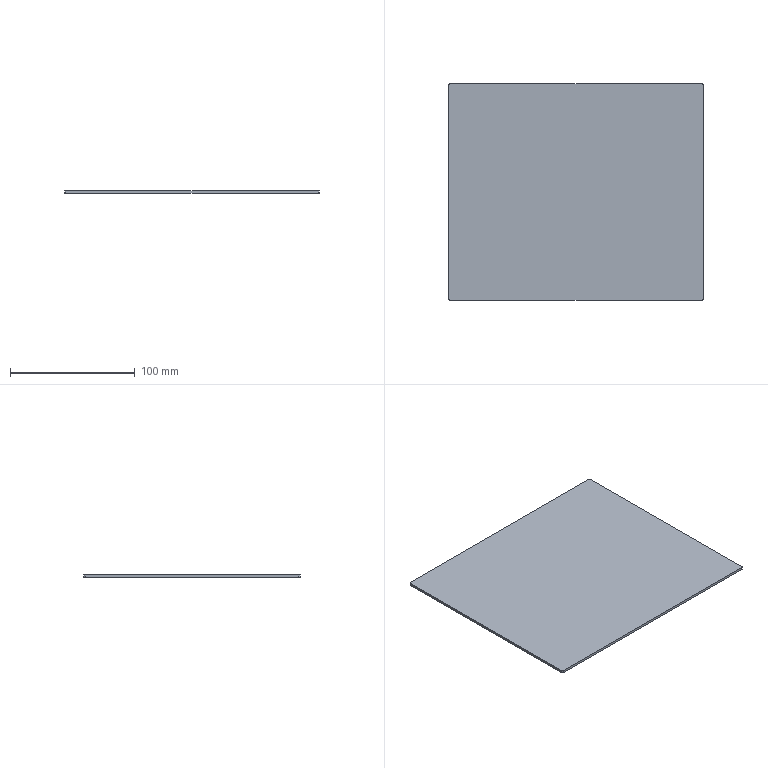Part | NX | features BREP 1 | 1 solid | 10 faces | box 204 x 173 x 2 mm | volume 70582 mm3 | plane 6 | cylinder 4 | commonest cylinder face diameters 2 x4
STEP:
#1=CARTESIAN_POINT('',(101.,86.5,-2.));
#2=VERTEX_POINT('',#1);
#3=CARTESIAN_POINT('',(-101.,86.5,-2.));
#4=VERTEX_POINT('',#3);
#5=CARTESIAN_POINT('',(-101.,86.5,-2.));
#6=DIRECTION('',(-1.,0.,0.));
#7=VECTOR('',#6,1000.);
#8=LINE('',#5,#7);
#9=EDGE_CURVE('',#2,#4,#8,.T.);
#10=ORIENTED_EDGE('',*,*,#9,.F.);
#11=CARTESIAN_POINT('',(102.,85.5,-2.));
#12=VERTEX_POINT('',#11);
#13=CARTESIAN_POINT('',(101.,85.5,-2.));
#14=DIRECTION('',(0.,0.,1.));
#15=DIRECTION('',(1.,0.,0.));
#16=AXIS2_PLACEMENT_3D('',#13,#14,#15);
#17=CIRCLE('',#16,1.);
#18=EDGE_CURVE('',#12,#2,#17,.T.);
#19=ORIENTED_EDGE('',*,*,#18,.F.);
#20=CARTESIAN_POINT('',(102.,-85.5,-2.));
#21=VERTEX_POINT('',#20);
#22=CARTESIAN_POINT('',(102.,-85.5,-2.));
#23=DIRECTION('',(0.,1.,0.));
#24=VECTOR('',#23,1000.);
#25=LINE('',#22,#24);
#26=EDGE_CURVE('',#21,#12,#25,.T.);
#27=ORIENTED_EDGE('',*,*,#26,.F.);
#28=CARTESIAN_POINT('',(101.,-86.5,-2.));
#29=VERTEX_POINT('',#28);
#30=CARTESIAN_POINT('',(101.,-85.5,-2.));
#31=DIRECTION('',(0.,0.,1.));
#32=DIRECTION('',(1.,0.,0.));
#33=AXIS2_PLACEMENT_3D('',#30,#31,#32);
#34=CIRCLE('',#33,1.);
#35=EDGE_CURVE('',#29,#21,#34,.T.);
#36=ORIENTED_EDGE('',*,*,#35,.F.);
#37=CARTESIAN_POINT('',(-101.,-86.5,-2.));
#38=VERTEX_POINT('',#37);
#39=CARTESIAN_POINT('',(-101.,-86.5,-2.));
#40=DIRECTION('',(1.,0.,0.));
#41=VECTOR('',#40,1000.);
#42=LINE('',#39,#41);
#43=EDGE_CURVE('',#38,#29,#42,.T.);
#44=ORIENTED_EDGE('',*,*,#43,.F.);
#45=CARTESIAN_POINT('',(-102.,-85.5,-2.));
#46=VERTEX_POINT('',#45);
#47=CARTESIAN_POINT('',(-101.,-85.5,-2.));
#48=DIRECTION('',(0.,0.,1.));
#49=DIRECTION('',(1.,0.,0.));
#50=AXIS2_PLACEMENT_3D('',#47,#48,#49);
#51=CIRCLE('',#50,1.);
#52=EDGE_CURVE('',#46,#38,#51,.T.);
#53=ORIENTED_EDGE('',*,*,#52,.F.);
#54=CARTESIAN_POINT('',(-102.,85.5,-2.));
#55=VERTEX_POINT('',#54);
#56=CARTESIAN_POINT('',(-102.,-85.5,-2.));
#57=DIRECTION('',(0.,-1.,0.));
#58=VECTOR('',#57,1000.);
#59=LINE('',#56,#58);
#60=EDGE_CURVE('',#55,#46,#59,.T.);
#61=ORIENTED_EDGE('',*,*,#60,.F.);
#62=CARTESIAN_POINT('',(-101.,85.5,-2.));
#63=DIRECTION('',(0.,0.,1.));
#64=DIRECTION('',(1.,0.,0.));
#65=AXIS2_PLACEMENT_3D('',#62,#63,#64);
#66=CIRCLE('',#65,1.);
#67=EDGE_CURVE('',#4,#55,#66,.T.);
#68=ORIENTED_EDGE('',*,*,#67,.F.);
#69=EDGE_LOOP('',(#10,#19,#27,#36,#44,#53,#61,#68));
#70=FACE_BOUND('',#69,.T.);
#71=CARTESIAN_POINT('',(-101.,-85.5,-2.));
#72=DIRECTION('',(0.,0.,1.));
#73=DIRECTION('',(-1.,0.,0.));
#74=AXIS2_PLACEMENT_3D('',#71,#72,#73);
#75=PLANE('',#74);
#76=ADVANCED_FACE('',(#70),#75,.F.);
#77=CARTESIAN_POINT('',(-101.,86.5,0.));
#78=VERTEX_POINT('',#77);
#79=CARTESIAN_POINT('',(-101.,86.5,-0.5));
#80=DIRECTION('',(0.,0.,-1.));
#81=VECTOR('',#80,1000.);
#82=LINE('',#79,#81);
#83=EDGE_CURVE('',#78,#4,#82,.T.);
#84=ORIENTED_EDGE('',*,*,#83,.F.);
#85=CARTESIAN_POINT('',(101.,86.5,0.));
#86=VERTEX_POINT('',#85);
#87=CARTESIAN_POINT('',(-101.,86.5,0.));
#88=DIRECTION('',(-1.,0.,0.));
#89=VECTOR('',#88,1000.);
#90=LINE('',#87,#89);
#91=EDGE_CURVE('',#86,#78,#90,.T.);
#92=ORIENTED_EDGE('',*,*,#91,.F.);
#93=CARTESIAN_POINT('',(101.,86.5,-0.5));
#94=DIRECTION('',(0.,0.,1.));
#95=VECTOR('',#94,1000.);
#96=LINE('',#93,#95);
#97=EDGE_CURVE('',#2,#86,#96,.T.);
#98=ORIENTED_EDGE('',*,*,#97,.F.);
#99=ORIENTED_EDGE('',*,*,#9,.T.);
#100=EDGE_LOOP('',(#84,#92,#98,#99));
#101=FACE_BOUND('',#100,.T.);
#102=CARTESIAN_POINT('',(-101.,86.5,-0.5));
#103=DIRECTION('',(0.,-1.,0.));
#104=DIRECTION('',(0.,0.,1.));
#105=AXIS2_PLACEMENT_3D('',#102,#103,#104);
#106=PLANE('',#105);
#107=ADVANCED_FACE('',(#101),#106,.F.);
#108=CARTESIAN_POINT('',(102.,85.5,0.));
#109=VERTEX_POINT('',#108);
#110=CARTESIAN_POINT('',(102.,85.5,-0.5));
#111=DIRECTION('',(0.,0.,-1.));
#112=VECTOR('',#111,1000.);
#113=LINE('',#110,#112);
#114=EDGE_CURVE('',#109,#12,#113,.T.);
#115=ORIENTED_EDGE('',*,*,#114,.F.);
#116=CARTESIAN_POINT('',(102.,-85.5,0.));
#117=VERTEX_POINT('',#116);
#118=CARTESIAN_POINT('',(102.,-85.5,0.));
#119=DIRECTION('',(0.,1.,0.));
#120=VECTOR('',#119,1000.);
#121=LINE('',#118,#120);
#122=EDGE_CURVE('',#117,#109,#121,.T.);
#123=ORIENTED_EDGE('',*,*,#122,.F.);
#124=CARTESIAN_POINT('',(102.,-85.5,-0.5));
#125=DIRECTION('',(0.,0.,1.));
#126=VECTOR('',#125,1000.);
#127=LINE('',#124,#126);
#128=EDGE_CURVE('',#21,#117,#127,.T.);
#129=ORIENTED_EDGE('',*,*,#128,.F.);
#130=ORIENTED_EDGE('',*,*,#26,.T.);
#131=EDGE_LOOP('',(#115,#123,#129,#130));
#132=FACE_BOUND('',#131,.T.);
#133=CARTESIAN_POINT('',(102.,-85.5,-0.5));
#134=DIRECTION('',(-1.,0.,0.));
#135=DIRECTION('',(0.,0.,-1.));
#136=AXIS2_PLACEMENT_3D('',#133,#134,#135);
#137=PLANE('',#136);
#138=ADVANCED_FACE('',(#132),#137,.F.);
#139=CARTESIAN_POINT('',(101.,-86.5,0.));
#140=VERTEX_POINT('',#139);
#141=CARTESIAN_POINT('',(101.,-86.5,-0.5));
#142=DIRECTION('',(0.,0.,-1.));
#143=VECTOR('',#142,1000.);
#144=LINE('',#141,#143);
#145=EDGE_CURVE('',#140,#29,#144,.T.);
#146=ORIENTED_EDGE('',*,*,#145,.F.);
#147=CARTESIAN_POINT('',(-101.,-86.5,0.));
#148=VERTEX_POINT('',#147);
#149=CARTESIAN_POINT('',(-101.,-86.5,0.));
#150=DIRECTION('',(1.,0.,0.));
#151=VECTOR('',#150,1000.);
#152=LINE('',#149,#151);
#153=EDGE_CURVE('',#148,#140,#152,.T.);
#154=ORIENTED_EDGE('',*,*,#153,.F.);
#155=CARTESIAN_POINT('',(-101.,-86.5,-0.5));
#156=DIRECTION('',(0.,0.,1.));
#157=VECTOR('',#156,1000.);
#158=LINE('',#155,#157);
#159=EDGE_CURVE('',#38,#148,#158,.T.);
#160=ORIENTED_EDGE('',*,*,#159,.F.);
#161=ORIENTED_EDGE('',*,*,#43,.T.);
#162=EDGE_LOOP('',(#146,#154,#160,#161));
#163=FACE_BOUND('',#162,.T.);
#164=CARTESIAN_POINT('',(-101.,-86.5,-0.5));
#165=DIRECTION('',(0.,1.,0.));
#166=DIRECTION('',(0.,0.,-1.));
#167=AXIS2_PLACEMENT_3D('',#164,#165,#166);
#168=PLANE('',#167);
#169=ADVANCED_FACE('',(#163),#168,.F.);
#170=CARTESIAN_POINT('',(-102.,-85.5,0.));
#171=VERTEX_POINT('',#170);
#172=CARTESIAN_POINT('',(-102.,-85.5,-0.5));
#173=DIRECTION('',(0.,0.,-1.));
#174=VECTOR('',#173,1000.);
#175=LINE('',#172,#174);
#176=EDGE_CURVE('',#171,#46,#175,.T.);
#177=ORIENTED_EDGE('',*,*,#176,.F.);
#178=CARTESIAN_POINT('',(-102.,85.5,0.));
#179=VERTEX_POINT('',#178);
#180=CARTESIAN_POINT('',(-102.,-85.5,0.));
#181=DIRECTION('',(0.,-1.,0.));
#182=VECTOR('',#181,1000.);
#183=LINE('',#180,#182);
#184=EDGE_CURVE('',#179,#171,#183,.T.);
#185=ORIENTED_EDGE('',*,*,#184,.F.);
#186=CARTESIAN_POINT('',(-102.,85.5,-0.5));
#187=DIRECTION('',(0.,0.,1.));
#188=VECTOR('',#187,1000.);
#189=LINE('',#186,#188);
#190=EDGE_CURVE('',#55,#179,#189,.T.);
#191=ORIENTED_EDGE('',*,*,#190,.F.);
#192=ORIENTED_EDGE('',*,*,#60,.T.);
#193=EDGE_LOOP('',(#177,#185,#191,#192));
#194=FACE_BOUND('',#193,.T.);
#195=CARTESIAN_POINT('',(-102.,-85.5,-0.5));
#196=DIRECTION('',(1.,0.,0.));
#197=DIRECTION('',(0.,0.,1.));
#198=AXIS2_PLACEMENT_3D('',#195,#196,#197);
#199=PLANE('',#198);
#200=ADVANCED_FACE('',(#194),#199,.F.);
#201=ORIENTED_EDGE('',*,*,#83,.T.);
#202=ORIENTED_EDGE('',*,*,#67,.T.);
#203=ORIENTED_EDGE('',*,*,#190,.T.);
#204=CARTESIAN_POINT('',(-101.,85.5,0.));
#205=DIRECTION('',(0.,0.,-1.));
#206=DIRECTION('',(1.,0.,0.));
#207=AXIS2_PLACEMENT_3D('',#204,#205,#206);
#208=CIRCLE('',#207,1.);
#209=EDGE_CURVE('',#179,#78,#208,.T.);
#210=ORIENTED_EDGE('',*,*,#209,.T.);
#211=EDGE_LOOP('',(#201,#202,#203,#210));
#212=FACE_BOUND('',#211,.T.);
#213=CARTESIAN_POINT('',(-101.,85.5,-0.5));
#214=DIRECTION('',(0.,0.,1.));
#215=DIRECTION('',(-1.,0.,0.));
#216=AXIS2_PLACEMENT_3D('',#213,#214,#215);
#217=CYLINDRICAL_SURFACE('',#216,1.);
#218=ADVANCED_FACE('',(#212),#217,.T.);
#219=ORIENTED_EDGE('',*,*,#91,.T.);
#220=ORIENTED_EDGE('',*,*,#209,.F.);
#221=ORIENTED_EDGE('',*,*,#184,.T.);
#222=CARTESIAN_POINT('',(-101.,-85.5,0.));
#223=DIRECTION('',(0.,0.,1.));
#224=DIRECTION('',(1.,0.,0.));
#225=AXIS2_PLACEMENT_3D('',#222,#223,#224);
#226=CIRCLE('',#225,1.);
#227=EDGE_CURVE('',#171,#148,#226,.T.);
#228=ORIENTED_EDGE('',*,*,#227,.T.);
#229=ORIENTED_EDGE('',*,*,#153,.T.);
#230=CARTESIAN_POINT('',(101.,-85.5,0.));
#231=DIRECTION('',(0.,0.,1.));
#232=DIRECTION('',(1.,0.,0.));
#233=AXIS2_PLACEMENT_3D('',#230,#231,#232);
#234=CIRCLE('',#233,1.);
#235=EDGE_CURVE('',#140,#117,#234,.T.);
#236=ORIENTED_EDGE('',*,*,#235,.T.);
#237=ORIENTED_EDGE('',*,*,#122,.T.);
#238=CARTESIAN_POINT('',(101.,85.5,0.));
#239=DIRECTION('',(0.,0.,1.));
#240=DIRECTION('',(1.,0.,0.));
#241=AXIS2_PLACEMENT_3D('',#238,#239,#240);
#242=CIRCLE('',#241,1.);
#243=EDGE_CURVE('',#109,#86,#242,.T.);
#244=ORIENTED_EDGE('',*,*,#243,.T.);
#245=EDGE_LOOP('',(#219,#220,#221,#228,#229,#236,#237,#244));
#246=FACE_BOUND('',#245,.T.);
#247=CARTESIAN_POINT('',(-101.,-85.5,0.));
#248=DIRECTION('',(0.,0.,1.));
#249=DIRECTION('',(-1.,0.,0.));
#250=AXIS2_PLACEMENT_3D('',#247,#248,#249);
#251=PLANE('',#250);
#252=ADVANCED_FACE('',(#246),#251,.T.);
#253=ORIENTED_EDGE('',*,*,#114,.T.);
#254=ORIENTED_EDGE('',*,*,#18,.T.);
#255=ORIENTED_EDGE('',*,*,#97,.T.);
#256=ORIENTED_EDGE('',*,*,#243,.F.);
#257=EDGE_LOOP('',(#253,#254,#255,#256));
#258=FACE_BOUND('',#257,.T.);
#259=CARTESIAN_POINT('',(101.,85.5,-0.5));
#260=DIRECTION('',(0.,0.,1.));
#261=DIRECTION('',(-1.,0.,0.));
#262=AXIS2_PLACEMENT_3D('',#259,#260,#261);
#263=CYLINDRICAL_SURFACE('',#262,1.);
#264=ADVANCED_FACE('',(#258),#263,.T.);
#265=ORIENTED_EDGE('',*,*,#145,.T.);
#266=ORIENTED_EDGE('',*,*,#35,.T.);
#267=ORIENTED_EDGE('',*,*,#128,.T.);
#268=ORIENTED_EDGE('',*,*,#235,.F.);
#269=EDGE_LOOP('',(#265,#266,#267,#268));
#270=FACE_BOUND('',#269,.T.);
#271=CARTESIAN_POINT('',(101.,-85.5,-0.5));
#272=DIRECTION('',(0.,0.,1.));
#273=DIRECTION('',(-1.,0.,0.));
#274=AXIS2_PLACEMENT_3D('',#271,#272,#273);
#275=CYLINDRICAL_SURFACE('',#274,1.);
#276=ADVANCED_FACE('',(#270),#275,.T.);
#277=ORIENTED_EDGE('',*,*,#176,.T.);
#278=ORIENTED_EDGE('',*,*,#52,.T.);
#279=ORIENTED_EDGE('',*,*,#159,.T.);
#280=ORIENTED_EDGE('',*,*,#227,.F.);
#281=EDGE_LOOP('',(#277,#278,#279,#280));
#282=FACE_BOUND('',#281,.T.);
#283=CARTESIAN_POINT('',(-101.,-85.5,-0.5));
#284=DIRECTION('',(0.,0.,1.));
#285=DIRECTION('',(-1.,0.,0.));
#286=AXIS2_PLACEMENT_3D('',#283,#284,#285);
#287=CYLINDRICAL_SURFACE('',#286,1.);
#288=ADVANCED_FACE('',(#282),#287,.T.);
#289=CLOSED_SHELL('',(#76,#107,#138,#169,#200,#218,#252,#264,#276,#288));
#290=MANIFOLD_SOLID_BREP('',#289);
#291=(LENGTH_UNIT()NAMED_UNIT(*)SI_UNIT(.MILLI.,.METRE.));
#292=UNCERTAINTY_MEASURE_WITH_UNIT(LENGTH_MEASURE(0.00001),#291,'','');
#293=(NAMED_UNIT(*)PLANE_ANGLE_UNIT()SI_UNIT($,.RADIAN.));
#294=(NAMED_UNIT(*)SI_UNIT($,.STERADIAN.)SOLID_ANGLE_UNIT());
#295=(GEOMETRIC_REPRESENTATION_CONTEXT(3)GLOBAL_UNCERTAINTY_ASSIGNED_CONTEXT((#292))GLOBAL_UNIT_ASSIGNED_CONTEXT((#291,#293,#294))REPRESENTATION_CONTEXT('',''));
#296=ADVANCED_BREP_SHAPE_REPRESENTATION('',(#290),#295);